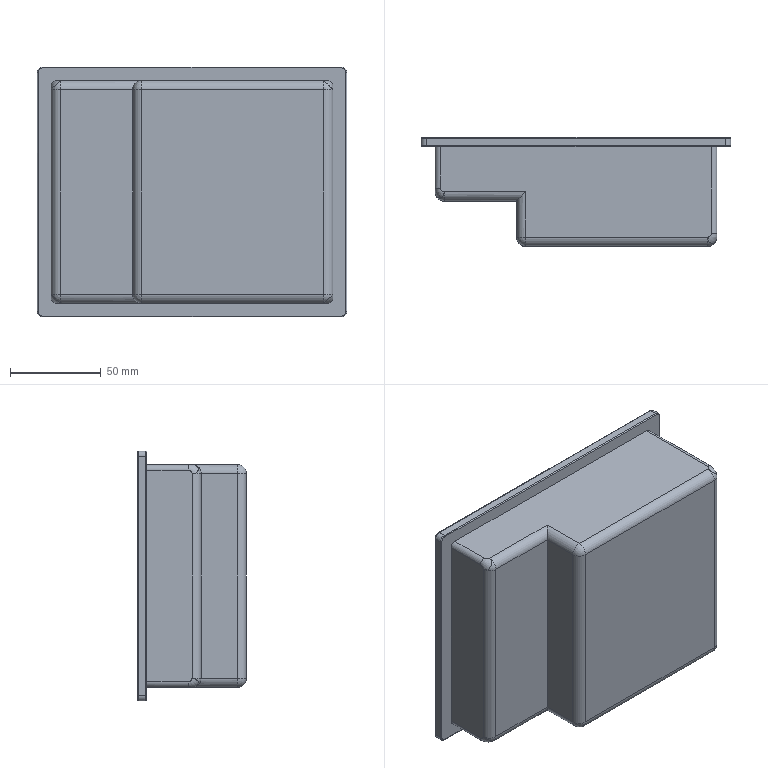Part | NX | 1 solid | 320 faces | box 171 x 60.05 x 138 mm | volume 1024818 mm3 | plane 275 | cylinder 27 | torus 8 | sphere 6 | spline 4 | commonest cylinder face diameters 10 x9 1 x8 6 x8 3 x2